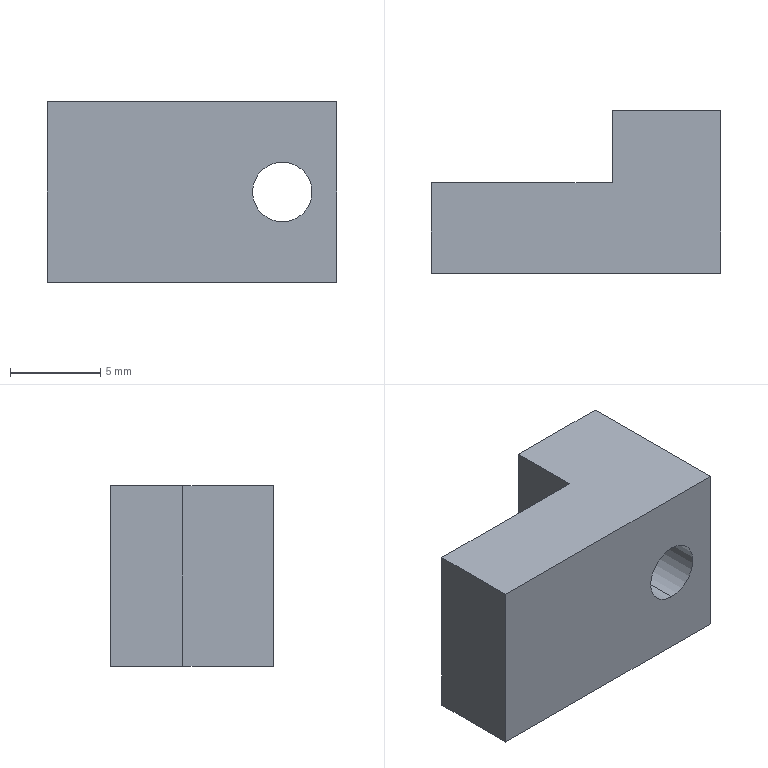Part | STEP file | limit block-1 | 1 solid | 13 faces | box 16 x 9 x 10 mm | volume 904.118 mm3 | plane 9 | cylinder 4 | commonest cylinder face diameters 3.3 x2 5 x2
STEP:
#1=CARTESIAN_POINT('',(0.,0.,0.));
#2=DIRECTION('',(0.,0.,1.));
#3=DIRECTION('',(1.,0.,0.));
#4=AXIS2_PLACEMENT_3D('',#1,#2,#3);
#5=CARTESIAN_POINT('',(5.5,-3.,7.5));
#6=VERTEX_POINT('',#5);
#7=CARTESIAN_POINT('',(5.5,0.,7.5));
#8=VERTEX_POINT('',#7);
#9=CARTESIAN_POINT('',(5.5,-3.,7.5));
#10=DIRECTION('',(0.,1.,0.));
#11=VECTOR('',#10,1.);
#12=LINE('',#9,#11);
#13=CARTESIAN_POINT('',(5.5,-3.,5.));
#14=DIRECTION('',(0.,1.,0.));
#15=DIRECTION('',(0.,0.,1.));
#16=AXIS2_PLACEMENT_3D('',#13,#14,#15);
#17=CYLINDRICAL_SURFACE('',#16,2.5);
#18=CARTESIAN_POINT('',(6.283,0.));
#19=DIRECTION('',(0.,1.));
#20=VECTOR('',#19,1.);
#21=LINE('',#18,#20);
#22=(GEOMETRIC_REPRESENTATION_CONTEXT(2)PARAMETRIC_REPRESENTATION_CONTEXT()REPRESENTATION_CONTEXT('',''));
#23=DEFINITIONAL_REPRESENTATION('',(#21),#22);
#24=PCURVE('',#17,#23);
#25=CARTESIAN_POINT('',(5.5,-3.,5.));
#26=DIRECTION('',(0.,1.,0.));
#27=DIRECTION('',(0.,0.,1.));
#28=AXIS2_PLACEMENT_3D('',#25,#26,#27);
#29=CYLINDRICAL_SURFACE('',#28,2.5);
#30=CARTESIAN_POINT('',(0.,0.));
#31=DIRECTION('',(0.,1.));
#32=VECTOR('',#31,1.);
#33=LINE('',#30,#32);
#34=(GEOMETRIC_REPRESENTATION_CONTEXT(2)PARAMETRIC_REPRESENTATION_CONTEXT()REPRESENTATION_CONTEXT('',''));
#35=DEFINITIONAL_REPRESENTATION('',(#33),#34);
#36=PCURVE('',#29,#35);
#37=SURFACE_CURVE('',#12,(#24,#36),.PCURVE_S1.);
#38=EDGE_CURVE('',#6,#8,#37,.T.);
#39=ORIENTED_EDGE('',*,*,#38,.T.);
#40=CARTESIAN_POINT('',(5.5,0.,2.5));
#41=VERTEX_POINT('',#40);
#42=CARTESIAN_POINT('',(5.5,0.,5.));
#43=DIRECTION('',(0.,1.,0.));
#44=DIRECTION('',(0.,0.,1.));
#45=AXIS2_PLACEMENT_3D('',#42,#43,#44);
#46=CIRCLE('',#45,2.5);
#47=CARTESIAN_POINT('',(0.,3.));
#48=DIRECTION('',(1.,0.));
#49=VECTOR('',#48,1.);
#50=LINE('',#47,#49);
#51=(GEOMETRIC_REPRESENTATION_CONTEXT(2)PARAMETRIC_REPRESENTATION_CONTEXT()REPRESENTATION_CONTEXT('',''));
#52=DEFINITIONAL_REPRESENTATION('',(#50),#51);
#53=PCURVE('',#17,#52);
#54=CARTESIAN_POINT('',(0.,0.,10.));
#55=DIRECTION('',(0.,-1.,0.));
#56=DIRECTION('',(0.,0.,-1.));
#57=AXIS2_PLACEMENT_3D('',#54,#55,#56);
#58=PLANE('',#57);
#59=CARTESIAN_POINT('',(2.5,5.5));
#60=CARTESIAN_POINT('',(2.5,9.83));
#61=CARTESIAN_POINT('',(6.25,7.665));
#62=CARTESIAN_POINT('',(10.,5.5));
#63=CARTESIAN_POINT('',(6.25,3.335));
#64=CARTESIAN_POINT('',(2.5,1.17));
#65=CARTESIAN_POINT('',(2.5,5.5));
#66=(BOUNDED_CURVE()B_SPLINE_CURVE(2,(#59,#60,#61,#62,#63,#64,#65),.UNSPECIFIED.,.T.,.F.)B_SPLINE_CURVE_WITH_KNOTS((1,2,2,2,2,1),(-2.094,0.,2.094,4.189,6.283,8.378),.UNSPECIFIED.)CURVE()GEOMETRIC_REPRESENTATION_ITEM()RATIONAL_B_SPLINE_CURVE((1.,0.5,1.,0.5,1.,0.5,1.))REPRESENTATION_ITEM(''));
#67=(GEOMETRIC_REPRESENTATION_CONTEXT(2)PARAMETRIC_REPRESENTATION_CONTEXT()REPRESENTATION_CONTEXT('',''));
#68=DEFINITIONAL_REPRESENTATION('',(#66),#67);
#69=PCURVE('',#58,#68);
#70=SURFACE_CURVE('',#46,(#53,#69),.PCURVE_S1.);
#71=EDGE_CURVE('',#41,#8,#70,.T.);
#72=ORIENTED_EDGE('',*,*,#71,.F.);
#73=CARTESIAN_POINT('',(5.5,-3.,2.5));
#74=VERTEX_POINT('',#73);
#75=CARTESIAN_POINT('',(5.5,-3.,2.5));
#76=DIRECTION('',(0.,1.,0.));
#77=VECTOR('',#76,1.);
#78=LINE('',#75,#77);
#79=CARTESIAN_POINT('',(3.142,0.));
#80=DIRECTION('',(0.,1.));
#81=VECTOR('',#80,1.);
#82=LINE('',#79,#81);
#83=(GEOMETRIC_REPRESENTATION_CONTEXT(2)PARAMETRIC_REPRESENTATION_CONTEXT()REPRESENTATION_CONTEXT('',''));
#84=DEFINITIONAL_REPRESENTATION('',(#82),#83);
#85=PCURVE('',#17,#84);
#86=CARTESIAN_POINT('',(3.142,0.));
#87=DIRECTION('',(0.,1.));
#88=VECTOR('',#87,1.);
#89=LINE('',#86,#88);
#90=(GEOMETRIC_REPRESENTATION_CONTEXT(2)PARAMETRIC_REPRESENTATION_CONTEXT()REPRESENTATION_CONTEXT('',''));
#91=DEFINITIONAL_REPRESENTATION('',(#89),#90);
#92=PCURVE('',#29,#91);
#93=SURFACE_CURVE('',#78,(#85,#92),.PCURVE_S1.);
#94=EDGE_CURVE('',#74,#41,#93,.T.);
#95=ORIENTED_EDGE('',*,*,#94,.F.);
#96=CARTESIAN_POINT('',(5.5,-3.,5.));
#97=DIRECTION('',(0.,1.,0.));
#98=DIRECTION('',(0.,0.,1.));
#99=AXIS2_PLACEMENT_3D('',#96,#97,#98);
#100=CIRCLE('',#99,2.5);
#101=CARTESIAN_POINT('',(0.,0.));
#102=DIRECTION('',(1.,0.));
#103=VECTOR('',#102,1.);
#104=LINE('',#101,#103);
#105=(GEOMETRIC_REPRESENTATION_CONTEXT(2)PARAMETRIC_REPRESENTATION_CONTEXT()REPRESENTATION_CONTEXT('',''));
#106=DEFINITIONAL_REPRESENTATION('',(#104),#105);
#107=PCURVE('',#17,#106);
#108=CARTESIAN_POINT('',(5.5,-3.,5.));
#109=DIRECTION('',(0.,1.,0.));
#110=DIRECTION('',(0.,0.,1.));
#111=AXIS2_PLACEMENT_3D('',#108,#109,#110);
#112=PLANE('',#111);
#113=CARTESIAN_POINT('',(0.,0.));
#114=DIRECTION('',(1.,0.));
#115=AXIS2_PLACEMENT_2D('',#113,#114);
#116=CIRCLE('',#115,2.5);
#117=(GEOMETRIC_REPRESENTATION_CONTEXT(2)PARAMETRIC_REPRESENTATION_CONTEXT()REPRESENTATION_CONTEXT('',''));
#118=DEFINITIONAL_REPRESENTATION('',(#116),#117);
#119=PCURVE('',#112,#118);
#120=SURFACE_CURVE('',#100,(#107,#119),.PCURVE_S1.);
#121=EDGE_CURVE('',#74,#6,#120,.T.);
#122=ORIENTED_EDGE('',*,*,#121,.T.);
#123=EDGE_LOOP('',(#39,#72,#95,#122));
#124=FACE_BOUND('',#123,.F.);
#125=ADVANCED_FACE('',(#124),#17,.F.);
#126=CARTESIAN_POINT('',(15.,-5.,6.65));
#127=VERTEX_POINT('',#126);
#128=CARTESIAN_POINT('',(15.,4.,6.65));
#129=VERTEX_POINT('',#128);
#130=CARTESIAN_POINT('',(15.,4.,6.65));
#131=DIRECTION('',(0.,1.,0.));
#132=VECTOR('',#131,1.);
#133=LINE('',#130,#132);
#134=CARTESIAN_POINT('',(15.,4.,5.));
#135=DIRECTION('',(0.,1.,0.));
#136=DIRECTION('',(0.,0.,1.));
#137=AXIS2_PLACEMENT_3D('',#134,#135,#136);
#138=CYLINDRICAL_SURFACE('',#137,1.65);
#139=CARTESIAN_POINT('',(6.283,0.));
#140=DIRECTION('',(0.,1.));
#141=VECTOR('',#140,1.);
#142=LINE('',#139,#141);
#143=(GEOMETRIC_REPRESENTATION_CONTEXT(2)PARAMETRIC_REPRESENTATION_CONTEXT()REPRESENTATION_CONTEXT('',''));
#144=DEFINITIONAL_REPRESENTATION('',(#142),#143);
#145=PCURVE('',#138,#144);
#146=CARTESIAN_POINT('',(15.,4.,5.));
#147=DIRECTION('',(0.,1.,0.));
#148=DIRECTION('',(0.,0.,1.));
#149=AXIS2_PLACEMENT_3D('',#146,#147,#148);
#150=CYLINDRICAL_SURFACE('',#149,1.65);
#151=CARTESIAN_POINT('',(0.,0.));
#152=DIRECTION('',(0.,1.));
#153=VECTOR('',#152,1.);
#154=LINE('',#151,#153);
#155=(GEOMETRIC_REPRESENTATION_CONTEXT(2)PARAMETRIC_REPRESENTATION_CONTEXT()REPRESENTATION_CONTEXT('',''));
#156=DEFINITIONAL_REPRESENTATION('',(#154),#155);
#157=PCURVE('',#150,#156);
#158=SURFACE_CURVE('',#133,(#145,#157),.PCURVE_S1.);
#159=EDGE_CURVE('',#127,#129,#158,.T.);
#160=ORIENTED_EDGE('',*,*,#159,.T.);
#161=CARTESIAN_POINT('',(15.,4.,3.35));
#162=VERTEX_POINT('',#161);
#163=CARTESIAN_POINT('',(15.,4.,5.));
#164=DIRECTION('',(0.,1.,0.));
#165=DIRECTION('',(0.,0.,1.));
#166=AXIS2_PLACEMENT_3D('',#163,#164,#165);
#167=CIRCLE('',#166,1.65);
#168=CARTESIAN_POINT('',(0.,0.));
#169=DIRECTION('',(1.,0.));
#170=VECTOR('',#169,1.);
#171=LINE('',#168,#170);
#172=(GEOMETRIC_REPRESENTATION_CONTEXT(2)PARAMETRIC_REPRESENTATION_CONTEXT()REPRESENTATION_CONTEXT('',''));
#173=DEFINITIONAL_REPRESENTATION('',(#171),#172);
#174=PCURVE('',#138,#173);
#175=CARTESIAN_POINT('',(12.,4.,10.));
#176=DIRECTION('',(0.,-1.,0.));
#177=DIRECTION('',(0.,0.,-1.));
#178=AXIS2_PLACEMENT_3D('',#175,#176,#177);
#179=PLANE('',#178);
#180=CARTESIAN_POINT('',(3.35,3.));
#181=CARTESIAN_POINT('',(3.35,5.858));
#182=CARTESIAN_POINT('',(5.825,4.429));
#183=CARTESIAN_POINT('',(8.3,3.));
#184=CARTESIAN_POINT('',(5.825,1.571));
#185=CARTESIAN_POINT('',(3.35,0.1421));
#186=CARTESIAN_POINT('',(3.35,3.));
#187=(BOUNDED_CURVE()B_SPLINE_CURVE(2,(#180,#181,#182,#183,#184,#185,#186),.UNSPECIFIED.,.T.,.F.)B_SPLINE_CURVE_WITH_KNOTS((1,2,2,2,2,1),(-2.094,0.,2.094,4.189,6.283,8.378),.UNSPECIFIED.)CURVE()GEOMETRIC_REPRESENTATION_ITEM()RATIONAL_B_SPLINE_CURVE((1.,0.5,1.,0.5,1.,0.5,1.))REPRESENTATION_ITEM(''));
#188=(GEOMETRIC_REPRESENTATION_CONTEXT(2)PARAMETRIC_REPRESENTATION_CONTEXT()REPRESENTATION_CONTEXT('',''));
#189=DEFINITIONAL_REPRESENTATION('',(#187),#188);
#190=PCURVE('',#179,#189);
#191=SURFACE_CURVE('',#167,(#174,#190),.PCURVE_S1.);
#192=EDGE_CURVE('',#162,#129,#191,.T.);
#193=ORIENTED_EDGE('',*,*,#192,.F.);
#194=CARTESIAN_POINT('',(15.,-5.,3.35));
#195=VERTEX_POINT('',#194);
#196=CARTESIAN_POINT('',(15.,4.,3.35));
#197=DIRECTION('',(0.,1.,0.));
#198=VECTOR('',#197,1.);
#199=LINE('',#196,#198);
#200=CARTESIAN_POINT('',(3.142,0.));
#201=DIRECTION('',(0.,1.));
#202=VECTOR('',#201,1.);
#203=LINE('',#200,#202);
#204=(GEOMETRIC_REPRESENTATION_CONTEXT(2)PARAMETRIC_REPRESENTATION_CONTEXT()REPRESENTATION_CONTEXT('',''));
#205=DEFINITIONAL_REPRESENTATION('',(#203),#204);
#206=PCURVE('',#138,#205);
#207=CARTESIAN_POINT('',(3.142,0.));
#208=DIRECTION('',(0.,1.));
#209=VECTOR('',#208,1.);
#210=LINE('',#207,#209);
#211=(GEOMETRIC_REPRESENTATION_CONTEXT(2)PARAMETRIC_REPRESENTATION_CONTEXT()REPRESENTATION_CONTEXT('',''));
#212=DEFINITIONAL_REPRESENTATION('',(#210),#211);
#213=PCURVE('',#150,#212);
#214=SURFACE_CURVE('',#199,(#206,#213),.PCURVE_S1.);
#215=EDGE_CURVE('',#195,#162,#214,.T.);
#216=ORIENTED_EDGE('',*,*,#215,.F.);
#217=CARTESIAN_POINT('',(15.,-5.,5.));
#218=DIRECTION('',(0.,1.,0.));
#219=DIRECTION('',(0.,0.,1.));
#220=AXIS2_PLACEMENT_3D('',#217,#218,#219);
#221=CIRCLE('',#220,1.65);
#222=CARTESIAN_POINT('',(0.,-9.));
#223=DIRECTION('',(1.,0.));
#224=VECTOR('',#223,1.);
#225=LINE('',#222,#224);
#226=(GEOMETRIC_REPRESENTATION_CONTEXT(2)PARAMETRIC_REPRESENTATION_CONTEXT()REPRESENTATION_CONTEXT('',''));
#227=DEFINITIONAL_REPRESENTATION('',(#225),#226);
#228=PCURVE('',#138,#227);
#229=CARTESIAN_POINT('',(18.,-5.,10.));
#230=DIRECTION('',(0.,1.,0.));
#231=DIRECTION('',(-1.,0.,0.));
#232=AXIS2_PLACEMENT_3D('',#229,#230,#231);
#233=PLANE('',#232);
#234=CARTESIAN_POINT('',(3.,-5.));
#235=DIRECTION('',(0.,1.));
#236=AXIS2_PLACEMENT_2D('',#234,#235);
#237=CIRCLE('',#236,1.65);
#238=(GEOMETRIC_REPRESENTATION_CONTEXT(2)PARAMETRIC_REPRESENTATION_CONTEXT()REPRESENTATION_CONTEXT('',''));
#239=DEFINITIONAL_REPRESENTATION('',(#237),#238);
#240=PCURVE('',#233,#239);
#241=SURFACE_CURVE('',#221,(#228,#240),.PCURVE_S1.);
#242=EDGE_CURVE('',#195,#127,#241,.T.);
#243=ORIENTED_EDGE('',*,*,#242,.T.);
#244=EDGE_LOOP('',(#160,#193,#216,#243));
#245=FACE_BOUND('',#244,.F.);
#246=ADVANCED_FACE('',(#245),#138,.F.);
#247=CARTESIAN_POINT('',(15.,-5.,5.));
#248=DIRECTION('',(0.,1.,0.));
#249=DIRECTION('',(0.,0.,1.));
#250=AXIS2_PLACEMENT_3D('',#247,#248,#249);
#251=CIRCLE('',#250,1.65);
#252=CARTESIAN_POINT('',(3.,-5.));
#253=DIRECTION('',(0.,1.));
#254=AXIS2_PLACEMENT_2D('',#252,#253);
#255=CIRCLE('',#254,1.65);
#256=(GEOMETRIC_REPRESENTATION_CONTEXT(2)PARAMETRIC_REPRESENTATION_CONTEXT()REPRESENTATION_CONTEXT('',''));
#257=DEFINITIONAL_REPRESENTATION('',(#255),#256);
#258=PCURVE('',#233,#257);
#259=CARTESIAN_POINT('',(0.,-9.));
#260=DIRECTION('',(1.,0.));
#261=VECTOR('',#260,1.);
#262=LINE('',#259,#261);
#263=(GEOMETRIC_REPRESENTATION_CONTEXT(2)PARAMETRIC_REPRESENTATION_CONTEXT()REPRESENTATION_CONTEXT('',''));
#264=DEFINITIONAL_REPRESENTATION('',(#262),#263);
#265=PCURVE('',#150,#264);
#266=SURFACE_CURVE('',#251,(#258,#265),.PCURVE_S1.);
#267=EDGE_CURVE('',#127,#195,#266,.T.);
#268=ORIENTED_EDGE('',*,*,#267,.T.);
#269=ORIENTED_EDGE('',*,*,#242,.T.);
#270=EDGE_LOOP('',(#268,#269));
#271=FACE_BOUND('',#270,.T.);
#272=CARTESIAN_POINT('',(2.,-5.,10.));
#273=VERTEX_POINT('',#272);
#274=CARTESIAN_POINT('',(18.,-5.,10.));
#275=VERTEX_POINT('',#274);
#276=CARTESIAN_POINT('',(18.,-5.,10.));
#277=DIRECTION('',(1.,0.,0.));
#278=VECTOR('',#277,1.);
#279=LINE('',#276,#278);
#280=CARTESIAN_POINT('',(0.,0.));
#281=DIRECTION('',(-1.,0.));
#282=VECTOR('',#281,1.);
#283=LINE('',#280,#282);
#284=(GEOMETRIC_REPRESENTATION_CONTEXT(2)PARAMETRIC_REPRESENTATION_CONTEXT()REPRESENTATION_CONTEXT('',''));
#285=DEFINITIONAL_REPRESENTATION('',(#283),#284);
#286=PCURVE('',#233,#285);
#287=CARTESIAN_POINT('',(0.,0.,10.));
#288=DIRECTION('',(0.,0.,-1.));
#289=DIRECTION('',(-1.,0.,0.));
#290=AXIS2_PLACEMENT_3D('',#287,#288,#289);
#291=PLANE('',#290);
#292=CARTESIAN_POINT('',(-18.,-5.));
#293=DIRECTION('',(-1.,0.));
#294=VECTOR('',#293,1.);
#295=LINE('',#292,#294);
#296=(GEOMETRIC_REPRESENTATION_CONTEXT(2)PARAMETRIC_REPRESENTATION_CONTEXT()REPRESENTATION_CONTEXT('',''));
#297=DEFINITIONAL_REPRESENTATION('',(#295),#296);
#298=PCURVE('',#291,#297);
#299=SURFACE_CURVE('',#279,(#286,#298),.PCURVE_S1.);
#300=EDGE_CURVE('',#273,#275,#299,.T.);
#301=ORIENTED_EDGE('',*,*,#300,.F.);
#302=CARTESIAN_POINT('',(2.,-5.,0.));
#303=VERTEX_POINT('',#302);
#304=CARTESIAN_POINT('',(2.,-5.,0.));
#305=DIRECTION('',(0.,0.,-1.));
#306=VECTOR('',#305,1.);
#307=LINE('',#304,#306);
#308=CARTESIAN_POINT('',(16.,-10.));
#309=DIRECTION('',(0.,-1.));
#310=VECTOR('',#309,1.);
#311=LINE('',#308,#310);
#312=(GEOMETRIC_REPRESENTATION_CONTEXT(2)PARAMETRIC_REPRESENTATION_CONTEXT()REPRESENTATION_CONTEXT('',''));
#313=DEFINITIONAL_REPRESENTATION('',(#311),#312);
#314=PCURVE('',#233,#313);
#315=CARTESIAN_POINT('',(2.,-5.,0.));
#316=DIRECTION('',(1.,0.,0.));
#317=DIRECTION('',(0.,0.,-1.));
#318=AXIS2_PLACEMENT_3D('',#315,#316,#317);
#319=PLANE('',#318);
#320=CARTESIAN_POINT('',(0.,0.));
#321=DIRECTION('',(1.,0.));
#322=VECTOR('',#321,1.);
#323=LINE('',#320,#322);
#324=(GEOMETRIC_REPRESENTATION_CONTEXT(2)PARAMETRIC_REPRESENTATION_CONTEXT()REPRESENTATION_CONTEXT('',''));
#325=DEFINITIONAL_REPRESENTATION('',(#323),#324);
#326=PCURVE('',#319,#325);
#327=SURFACE_CURVE('',#307,(#314,#326),.PCURVE_S1.);
#328=EDGE_CURVE('',#273,#303,#327,.T.);
#329=ORIENTED_EDGE('',*,*,#328,.T.);
#330=CARTESIAN_POINT('',(18.,-5.,0.));
#331=VERTEX_POINT('',#330);
#332=CARTESIAN_POINT('',(18.,-5.,0.));
#333=DIRECTION('',(1.,0.,0.));
#334=VECTOR('',#333,1.);
#335=LINE('',#332,#334);
#336=CARTESIAN_POINT('',(0.,-10.));
#337=DIRECTION('',(-1.,0.));
#338=VECTOR('',#337,1.);
#339=LINE('',#336,#338);
#340=(GEOMETRIC_REPRESENTATION_CONTEXT(2)PARAMETRIC_REPRESENTATION_CONTEXT()REPRESENTATION_CONTEXT('',''));
#341=DEFINITIONAL_REPRESENTATION('',(#339),#340);
#342=PCURVE('',#233,#341);
#343=CARTESIAN_POINT('',(0.,0.,0.));
#344=DIRECTION('',(0.,0.,-1.));
#345=DIRECTION('',(-1.,0.,0.));
#346=AXIS2_PLACEMENT_3D('',#343,#344,#345);
#347=PLANE('',#346);
#348=CARTESIAN_POINT('',(-18.,-5.));
#349=DIRECTION('',(-1.,0.));
#350=VECTOR('',#349,1.);
#351=LINE('',#348,#350);
#352=(GEOMETRIC_REPRESENTATION_CONTEXT(2)PARAMETRIC_REPRESENTATION_CONTEXT()REPRESENTATION_CONTEXT('',''));
#353=DEFINITIONAL_REPRESENTATION('',(#351),#352);
#354=PCURVE('',#347,#353);
#355=SURFACE_CURVE('',#335,(#342,#354),.PCURVE_S1.);
#356=EDGE_CURVE('',#303,#331,#355,.T.);
#357=ORIENTED_EDGE('',*,*,#356,.T.);
#358=CARTESIAN_POINT('',(18.,-5.,10.));
#359=DIRECTION('',(0.,0.,-1.));
#360=VECTOR('',#359,1.);
#361=LINE('',#358,#360);
#362=CARTESIAN_POINT('',(0.,0.));
#363=DIRECTION('',(0.,-1.));
#364=VECTOR('',#363,1.);
#365=LINE('',#362,#364);
#366=(GEOMETRIC_REPRESENTATION_CONTEXT(2)PARAMETRIC_REPRESENTATION_CONTEXT()REPRESENTATION_CONTEXT('',''));
#367=DEFINITIONAL_REPRESENTATION('',(#365),#366);
#368=PCURVE('',#233,#367);
#369=CARTESIAN_POINT('',(18.,4.,10.));
#370=DIRECTION('',(-1.,0.,0.));
#371=DIRECTION('',(0.,0.,1.));
#372=AXIS2_PLACEMENT_3D('',#369,#370,#371);
#373=PLANE('',#372);
#374=CARTESIAN_POINT('',(0.,-9.));
#375=DIRECTION('',(-1.,0.));
#376=VECTOR('',#375,1.);
#377=LINE('',#374,#376);
#378=(GEOMETRIC_REPRESENTATION_CONTEXT(2)PARAMETRIC_REPRESENTATION_CONTEXT()REPRESENTATION_CONTEXT('',''));
#379=DEFINITIONAL_REPRESENTATION('',(#377),#378);
#380=PCURVE('',#373,#379);
#381=SURFACE_CURVE('',#361,(#368,#380),.PCURVE_S1.);
#382=EDGE_CURVE('',#275,#331,#381,.T.);
#383=ORIENTED_EDGE('',*,*,#382,.F.);
#384=EDGE_LOOP('',(#301,#329,#357,#383));
#385=FACE_BOUND('',#384,.T.);
#386=ADVANCED_FACE('',(#271,#385),#233,.F.);
#387=CARTESIAN_POINT('',(18.,4.,0.));
#388=VERTEX_POINT('',#387);
#389=CARTESIAN_POINT('',(18.,4.,0.));
#390=DIRECTION('',(0.,1.,0.));
#391=VECTOR('',#390,1.);
#392=LINE('',#389,#391);
#393=CARTESIAN_POINT('',(-10.,0.));
#394=DIRECTION('',(0.,1.));
#395=VECTOR('',#394,1.);
#396=LINE('',#393,#395);
#397=(GEOMETRIC_REPRESENTATION_CONTEXT(2)PARAMETRIC_REPRESENTATION_CONTEXT()REPRESENTATION_CONTEXT('',''));
#398=DEFINITIONAL_REPRESENTATION('',(#396),#397);
#399=PCURVE('',#373,#398);
#400=CARTESIAN_POINT('',(-18.,4.));
#401=DIRECTION('',(0.,1.));
#402=VECTOR('',#401,1.);
#403=LINE('',#400,#402);
#404=(GEOMETRIC_REPRESENTATION_CONTEXT(2)PARAMETRIC_REPRESENTATION_CONTEXT()REPRESENTATION_CONTEXT('',''));
#405=DEFINITIONAL_REPRESENTATION('',(#403),#404);
#406=PCURVE('',#347,#405);
#407=SURFACE_CURVE('',#392,(#399,#406),.PCURVE_S1.);
#408=EDGE_CURVE('',#331,#388,#407,.T.);
#409=ORIENTED_EDGE('',*,*,#408,.T.);
#410=CARTESIAN_POINT('',(18.,4.,10.));
#411=VERTEX_POINT('',#410);
#412=CARTESIAN_POINT('',(18.,4.,10.));
#413=DIRECTION('',(0.,0.,-1.));
#414=VECTOR('',#413,1.);
#415=LINE('',#412,#414);
#416=CARTESIAN_POINT('',(0.,0.));
#417=DIRECTION('',(-1.,0.));
#418=VECTOR('',#417,1.);
#419=LINE('',#416,#418);
#420=(GEOMETRIC_REPRESENTATION_CONTEXT(2)PARAMETRIC_REPRESENTATION_CONTEXT()REPRESENTATION_CONTEXT('',''));
#421=DEFINITIONAL_REPRESENTATION('',(#419),#420);
#422=PCURVE('',#373,#421);
#423=CARTESIAN_POINT('',(0.,6.));
#424=DIRECTION('',(1.,0.));
#425=VECTOR('',#424,1.);
#426=LINE('',#423,#425);
#427=(GEOMETRIC_REPRESENTATION_CONTEXT(2)PARAMETRIC_REPRESENTATION_CONTEXT()REPRESENTATION_CONTEXT('',''));
#428=DEFINITIONAL_REPRESENTATION('',(#426),#427);
#429=PCURVE('',#179,#428);
#430=SURFACE_CURVE('',#415,(#422,#429),.PCURVE_S1.);
#431=EDGE_CURVE('',#411,#388,#430,.T.);
#432=ORIENTED_EDGE('',*,*,#431,.F.);
#433=CARTESIAN_POINT('',(18.,4.,10.));
#434=DIRECTION('',(0.,1.,0.));
#435=VECTOR('',#434,1.);
#436=LINE('',#433,#435);
#437=CARTESIAN_POINT('',(0.,0.));
#438=DIRECTION('',(0.,1.));
#439=VECTOR('',#438,1.);
#440=LINE('',#437,#439);
#441=(GEOMETRIC_REPRESENTATION_CONTEXT(2)PARAMETRIC_REPRESENTATION_CONTEXT()REPRESENTATION_CONTEXT('',''));
#442=DEFINITIONAL_REPRESENTATION('',(#440),#441);
#443=PCURVE('',#373,#442);
#444=CARTESIAN_POINT('',(-18.,4.));
#445=DIRECTION('',(0.,1.));
#446=VECTOR('',#445,1.);
#447=LINE('',#444,#446);
#448=(GEOMETRIC_REPRESENTATION_CONTEXT(2)PARAMETRIC_REPRESENTATION_CONTEXT()REPRESENTATION_CONTEXT('',''));
#449=DEFINITIONAL_REPRESENTATION('',(#447),#448);
#450=PCURVE('',#291,#449);
#451=SURFACE_CURVE('',#436,(#443,#450),.PCURVE_S1.);
#452=EDGE_CURVE('',#275,#411,#451,.T.);
#453=ORIENTED_EDGE('',*,*,#452,.F.);
#454=ORIENTED_EDGE('',*,*,#382,.T.);
#455=EDGE_LOOP('',(#409,#432,#453,#454));
#456=FACE_BOUND('',#455,.T.);
#457=ADVANCED_FACE('',(#456),#373,.F.);
#458=CARTESIAN_POINT('',(15.,4.,5.));
#459=DIRECTION('',(0.,1.,0.));
#460=DIRECTION('',(0.,0.,1.));
#461=AXIS2_PLACEMENT_3D('',#458,#459,#460);
#462=CIRCLE('',#461,1.65);
#463=CARTESIAN_POINT('',(3.35,3.));
#464=CARTESIAN_POINT('',(3.35,5.858));
#465=CARTESIAN_POINT('',(5.825,4.429));
#466=CARTESIAN_POINT('',(8.3,3.));
#467=CARTESIAN_POINT('',(5.825,1.571));
#468=CARTESIAN_POINT('',(3.35,0.1421));
#469=CARTESIAN_POINT('',(3.35,3.));
#470=(BOUNDED_CURVE()B_SPLINE_CURVE(2,(#463,#464,#465,#466,#467,#468,#469),.UNSPECIFIED.,.T.,.F.)B_SPLINE_CURVE_WITH_KNOTS((1,2,2,2,2,1),(-2.094,0.,2.094,4.189,6.283,8.378),.UNSPECIFIED.)CURVE()GEOMETRIC_REPRESENTATION_ITEM()RATIONAL_B_SPLINE_CURVE((1.,0.5,1.,0.5,1.,0.5,1.))REPRESENTATION_ITEM(''));
#471=(GEOMETRIC_REPRESENTATION_CONTEXT(2)PARAMETRIC_REPRESENTATION_CONTEXT()REPRESENTATION_CONTEXT('',''));
#472=DEFINITIONAL_REPRESENTATION('',(#470),#471);
#473=PCURVE('',#179,#472);
#474=CARTESIAN_POINT('',(0.,0.));
#475=DIRECTION('',(1.,0.));
#476=VECTOR('',#475,1.);
#477=LINE('',#474,#476);
#478=(GEOMETRIC_REPRESENTATION_CONTEXT(2)PARAMETRIC_REPRESENTATION_CONTEXT()REPRESENTATION_CONTEXT('',''));
#479=DEFINITIONAL_REPRESENTATION('',(#477),#478);
#480=PCURVE('',#150,#479);
#481=SURFACE_CURVE('',#462,(#473,#480),.PCURVE_S1.);
#482=EDGE_CURVE('',#129,#162,#481,.T.);
#483=ORIENTED_EDGE('',*,*,#482,.F.);
#484=ORIENTED_EDGE('',*,*,#192,.F.);
#485=EDGE_LOOP('',(#483,#484));
#486=FACE_BOUND('',#485,.T.);
#487=CARTESIAN_POINT('',(12.,4.,0.));
#488=VERTEX_POINT('',#487);
#489=CARTESIAN_POINT('',(12.,4.,0.));
#490=DIRECTION('',(-1.,0.,0.));
#491=VECTOR('',#490,1.);
#492=LINE('',#489,#491);
#493=CARTESIAN_POINT('',(10.,0.));
#494=DIRECTION('',(0.,-1.));
#495=VECTOR('',#494,1.);
#496=LINE('',#493,#495);
#497=(GEOMETRIC_REPRESENTATION_CONTEXT(2)PARAMETRIC_REPRESENTATION_CONTEXT()REPRESENTATION_CONTEXT('',''));
#498=DEFINITIONAL_REPRESENTATION('',(#496),#497);
#499=PCURVE('',#179,#498);
#500=CARTESIAN_POINT('',(-12.,4.));
#501=DIRECTION('',(1.,0.));
#502=VECTOR('',#501,1.);
#503=LINE('',#500,#502);
#504=(GEOMETRIC_REPRESENTATION_CONTEXT(2)PARAMETRIC_REPRESENTATION_CONTEXT()REPRESENTATION_CONTEXT('',''));
#505=DEFINITIONAL_REPRESENTATION('',(#503),#504);
#506=PCURVE('',#347,#505);
#507=SURFACE_CURVE('',#492,(#499,#506),.PCURVE_S1.);
#508=EDGE_CURVE('',#388,#488,#507,.T.);
#509=ORIENTED_EDGE('',*,*,#508,.T.);
#510=CARTESIAN_POINT('',(12.,4.,10.));
#511=VERTEX_POINT('',#510);
#512=CARTESIAN_POINT('',(12.,4.,10.));
#513=DIRECTION('',(0.,0.,-1.));
#514=VECTOR('',#513,1.);
#515=LINE('',#512,#514);
#516=CARTESIAN_POINT('',(0.,0.));
#517=DIRECTION('',(1.,0.));
#518=VECTOR('',#517,1.);
#519=LINE('',#516,#518);
#520=(GEOMETRIC_REPRESENTATION_CONTEXT(2)PARAMETRIC_REPRESENTATION_CONTEXT()REPRESENTATION_CONTEXT('',''));
#521=DEFINITIONAL_REPRESENTATION('',(#519),#520);
#522=PCURVE('',#179,#521);
#523=CARTESIAN_POINT('',(12.,0.,10.));
#524=DIRECTION('',(1.,0.,0.));
#525=DIRECTION('',(0.,0.,-1.));
#526=AXIS2_PLACEMENT_3D('',#523,#524,#525);
#527=PLANE('',#526);
#528=CARTESIAN_POINT('',(0.,4.));
#529=DIRECTION('',(1.,0.));
#530=VECTOR('',#529,1.);
#531=LINE('',#528,#530);
#532=(GEOMETRIC_REPRESENTATION_CONTEXT(2)PARAMETRIC_REPRESENTATION_CONTEXT()REPRESENTATION_CONTEXT('',''));
#533=DEFINITIONAL_REPRESENTATION('',(#531),#532);
#534=PCURVE('',#527,#533);
#535=SURFACE_CURVE('',#515,(#522,#534),.PCURVE_S1.);
#536=EDGE_CURVE('',#511,#488,#535,.T.);
#537=ORIENTED_EDGE('',*,*,#536,.F.);
#538=CARTESIAN_POINT('',(12.,4.,10.));
#539=DIRECTION('',(-1.,0.,0.));
#540=VECTOR('',#539,1.);
#541=LINE('',#538,#540);
#542=CARTESIAN_POINT('',(0.,0.));
#543=DIRECTION('',(0.,-1.));
#544=VECTOR('',#543,1.);
#545=LINE('',#542,#544);
#546=(GEOMETRIC_REPRESENTATION_CONTEXT(2)PARAMETRIC_REPRESENTATION_CONTEXT()REPRESENTATION_CONTEXT('',''));
#547=DEFINITIONAL_REPRESENTATION('',(#545),#546);
#548=PCURVE('',#179,#547);
#549=CARTESIAN_POINT('',(-12.,4.));
#550=DIRECTION('',(1.,0.));
#551=VECTOR('',#550,1.);
#552=LINE('',#549,#551);
#553=(GEOMETRIC_REPRESENTATION_CONTEXT(2)PARAMETRIC_REPRESENTATION_CONTEXT()REPRESENTATION_CONTEXT('',''));
#554=DEFINITIONAL_REPRESENTATION('',(#552),#553);
#555=PCURVE('',#291,#554);
#556=SURFACE_CURVE('',#541,(#548,#555),.PCURVE_S1.);
#557=EDGE_CURVE('',#411,#511,#556,.T.);
#558=ORIENTED_EDGE('',*,*,#557,.F.);
#559=ORIENTED_EDGE('',*,*,#431,.T.);
#560=EDGE_LOOP('',(#509,#537,#558,#559));
#561=FACE_BOUND('',#560,.T.);
#562=ADVANCED_FACE('',(#486,#561),#179,.F.);
#563=CARTESIAN_POINT('',(12.,0.,0.));
#564=VERTEX_POINT('',#563);
#565=CARTESIAN_POINT('',(12.,0.,0.));
#566=DIRECTION('',(0.,-1.,0.));
#567=VECTOR('',#566,1.);
#568=LINE('',#565,#567);
#569=CARTESIAN_POINT('',(10.,0.));
#570=DIRECTION('',(0.,-1.));
#571=VECTOR('',#570,1.);
#572=LINE('',#569,#571);
#573=(GEOMETRIC_REPRESENTATION_CONTEXT(2)PARAMETRIC_REPRESENTATION_CONTEXT()REPRESENTATION_CONTEXT('',''));
#574=DEFINITIONAL_REPRESENTATION('',(#572),#573);
#575=PCURVE('',#527,#574);
#576=CARTESIAN_POINT('',(-12.,0.));
#577=DIRECTION('',(0.,-1.));
#578=VECTOR('',#577,1.);
#579=LINE('',#576,#578);
#580=(GEOMETRIC_REPRESENTATION_CONTEXT(2)PARAMETRIC_REPRESENTATION_CONTEXT()REPRESENTATION_CONTEXT('',''));
#581=DEFINITIONAL_REPRESENTATION('',(#579),#580);
#582=PCURVE('',#347,#581);
#583=SURFACE_CURVE('',#568,(#575,#582),.PCURVE_S1.);
#584=EDGE_CURVE('',#488,#564,#583,.T.);
#585=ORIENTED_EDGE('',*,*,#584,.T.);
#586=CARTESIAN_POINT('',(12.,0.,10.));
#587=VERTEX_POINT('',#586);
#588=CARTESIAN_POINT('',(12.,0.,10.));
#589=DIRECTION('',(0.,0.,-1.));
#590=VECTOR('',#589,1.);
#591=LINE('',#588,#590);
#592=CARTESIAN_POINT('',(0.,0.));
#593=DIRECTION('',(1.,0.));
#594=VECTOR('',#593,1.);
#595=LINE('',#592,#594);
#596=(GEOMETRIC_REPRESENTATION_CONTEXT(2)PARAMETRIC_REPRESENTATION_CONTEXT()REPRESENTATION_CONTEXT('',''));
#597=DEFINITIONAL_REPRESENTATION('',(#595),#596);
#598=PCURVE('',#527,#597);
#599=CARTESIAN_POINT('',(0.,12.));
#600=DIRECTION('',(1.,0.));
#601=VECTOR('',#600,1.);
#602=LINE('',#599,#601);
#603=(GEOMETRIC_REPRESENTATION_CONTEXT(2)PARAMETRIC_REPRESENTATION_CONTEXT()REPRESENTATION_CONTEXT('',''));
#604=DEFINITIONAL_REPRESENTATION('',(#602),#603);
#605=PCURVE('',#58,#604);
#606=SURFACE_CURVE('',#591,(#598,#605),.PCURVE_S1.);
#607=EDGE_CURVE('',#587,#564,#606,.T.);
#608=ORIENTED_EDGE('',*,*,#607,.F.);
#609=CARTESIAN_POINT('',(12.,0.,10.));
#610=DIRECTION('',(0.,-1.,0.));
#611=VECTOR('',#610,1.);
#612=LINE('',#609,#611);
#613=CARTESIAN_POINT('',(0.,0.));
#614=DIRECTION('',(0.,-1.));
#615=VECTOR('',#614,1.);
#616=LINE('',#613,#615);
#617=(GEOMETRIC_REPRESENTATION_CONTEXT(2)PARAMETRIC_REPRESENTATION_CONTEXT()REPRESENTATION_CONTEXT('',''));
#618=DEFINITIONAL_REPRESENTATION('',(#616),#617);
#619=PCURVE('',#527,#618);
#620=CARTESIAN_POINT('',(-12.,0.));
#621=DIRECTION('',(0.,-1.));
#622=VECTOR('',#621,1.);
#623=LINE('',#620,#622);
#624=(GEOMETRIC_REPRESENTATION_CONTEXT(2)PARAMETRIC_REPRESENTATION_CONTEXT()REPRESENTATION_CONTEXT('',''));
#625=DEFINITIONAL_REPRESENTATION('',(#623),#624);
#626=PCURVE('',#291,#625);
#627=SURFACE_CURVE('',#612,(#619,#626),.PCURVE_S1.);
#628=EDGE_CURVE('',#511,#587,#627,.T.);
#629=ORIENTED_EDGE('',*,*,#628,.F.);
#630=ORIENTED_EDGE('',*,*,#536,.T.);
#631=EDGE_LOOP('',(#585,#608,#629,#630));
#632=FACE_BOUND('',#631,.T.);
#633=ADVANCED_FACE('',(#632),#527,.F.);
#634=CARTESIAN_POINT('',(5.5,0.,5.));
#635=DIRECTION('',(0.,1.,0.));
#636=DIRECTION('',(0.,0.,1.));
#637=AXIS2_PLACEMENT_3D('',#634,#635,#636);
#638=CIRCLE('',#637,2.5);
#639=CARTESIAN_POINT('',(2.5,5.5));
#640=CARTESIAN_POINT('',(2.5,9.83));
#641=CARTESIAN_POINT('',(6.25,7.665));
#642=CARTESIAN_POINT('',(10.,5.5));
#643=CARTESIAN_POINT('',(6.25,3.335));
#644=CARTESIAN_POINT('',(2.5,1.17));
#645=CARTESIAN_POINT('',(2.5,5.5));
#646=(BOUNDED_CURVE()B_SPLINE_CURVE(2,(#639,#640,#641,#642,#643,#644,#645),.UNSPECIFIED.,.T.,.F.)B_SPLINE_CURVE_WITH_KNOTS((1,2,2,2,2,1),(-2.094,0.,2.094,4.189,6.283,8.378),.UNSPECIFIED.)CURVE()GEOMETRIC_REPRESENTATION_ITEM()RATIONAL_B_SPLINE_CURVE((1.,0.5,1.,0.5,1.,0.5,1.))REPRESENTATION_ITEM(''));
#647=(GEOMETRIC_REPRESENTATION_CONTEXT(2)PARAMETRIC_REPRESENTATION_CONTEXT()REPRESENTATION_CONTEXT('',''));
#648=DEFINITIONAL_REPRESENTATION('',(#646),#647);
#649=PCURVE('',#58,#648);
#650=CARTESIAN_POINT('',(0.,3.));
#651=DIRECTION('',(1.,0.));
#652=VECTOR('',#651,1.);
#653=LINE('',#650,#652);
#654=(GEOMETRIC_REPRESENTATION_CONTEXT(2)PARAMETRIC_REPRESENTATION_CONTEXT()REPRESENTATION_CONTEXT('',''));
#655=DEFINITIONAL_REPRESENTATION('',(#653),#654);
#656=PCURVE('',#29,#655);
#657=SURFACE_CURVE('',#638,(#649,#656),.PCURVE_S1.);
#658=EDGE_CURVE('',#8,#41,#657,.T.);
#659=ORIENTED_EDGE('',*,*,#658,.F.);
#660=ORIENTED_EDGE('',*,*,#71,.F.);
#661=EDGE_LOOP('',(#659,#660));
#662=FACE_BOUND('',#661,.T.);
#663=CARTESIAN_POINT('',(2.,0.,0.));
#664=VERTEX_POINT('',#663);
#665=CARTESIAN_POINT('',(0.,0.,0.));
#666=DIRECTION('',(-1.,0.,0.));
#667=VECTOR('',#666,1.);
#668=LINE('',#665,#667);
#669=CARTESIAN_POINT('',(10.,0.));
#670=DIRECTION('',(0.,-1.));
#671=VECTOR('',#670,1.);
#672=LINE('',#669,#671);
#673=(GEOMETRIC_REPRESENTATION_CONTEXT(2)PARAMETRIC_REPRESENTATION_CONTEXT()REPRESENTATION_CONTEXT('',''));
#674=DEFINITIONAL_REPRESENTATION('',(#672),#673);
#675=PCURVE('',#58,#674);
#676=CARTESIAN_POINT('',(0.,0.));
#677=DIRECTION('',(1.,0.));
#678=VECTOR('',#677,1.);
#679=LINE('',#676,#678);
#680=(GEOMETRIC_REPRESENTATION_CONTEXT(2)PARAMETRIC_REPRESENTATION_CONTEXT()REPRESENTATION_CONTEXT('',''));
#681=DEFINITIONAL_REPRESENTATION('',(#679),#680);
#682=PCURVE('',#347,#681);
#683=SURFACE_CURVE('',#668,(#675,#682),.PCURVE_S1.);
#684=EDGE_CURVE('',#564,#664,#683,.T.);
#685=ORIENTED_EDGE('',*,*,#684,.T.);
#686=CARTESIAN_POINT('',(2.,0.,10.));
#687=VERTEX_POINT('',#686);
#688=CARTESIAN_POINT('',(2.,0.,0.));
#689=DIRECTION('',(0.,0.,-1.));
#690=VECTOR('',#689,1.);
#691=LINE('',#688,#690);
#692=CARTESIAN_POINT('',(10.,2.));
#693=DIRECTION('',(1.,0.));
#694=VECTOR('',#693,1.);
#695=LINE('',#692,#694);
#696=(GEOMETRIC_REPRESENTATION_CONTEXT(2)PARAMETRIC_REPRESENTATION_CONTEXT()REPRESENTATION_CONTEXT('',''));
#697=DEFINITIONAL_REPRESENTATION('',(#695),#696);
#698=PCURVE('',#58,#697);
#699=CARTESIAN_POINT('',(0.,5.));
#700=DIRECTION('',(1.,0.));
#701=VECTOR('',#700,1.);
#702=LINE('',#699,#701);
#703=(GEOMETRIC_REPRESENTATION_CONTEXT(2)PARAMETRIC_REPRESENTATION_CONTEXT()REPRESENTATION_CONTEXT('',''));
#704=DEFINITIONAL_REPRESENTATION('',(#702),#703);
#705=PCURVE('',#319,#704);
#706=SURFACE_CURVE('',#691,(#698,#705),.PCURVE_S1.);
#707=EDGE_CURVE('',#687,#664,#706,.T.);
#708=ORIENTED_EDGE('',*,*,#707,.F.);
#709=CARTESIAN_POINT('',(0.,0.,10.));
#710=DIRECTION('',(-1.,0.,0.));
#711=VECTOR('',#710,1.);
#712=LINE('',#709,#711);
#713=CARTESIAN_POINT('',(0.,0.));
#714=DIRECTION('',(0.,-1.));
#715=VECTOR('',#714,1.);
#716=LINE('',#713,#715);
#717=(GEOMETRIC_REPRESENTATION_CONTEXT(2)PARAMETRIC_REPRESENTATION_CONTEXT()REPRESENTATION_CONTEXT('',''));
#718=DEFINITIONAL_REPRESENTATION('',(#716),#717);
#719=PCURVE('',#58,#718);
#720=CARTESIAN_POINT('',(0.,0.));
#721=DIRECTION('',(1.,0.));
#722=VECTOR('',#721,1.);
#723=LINE('',#720,#722);
#724=(GEOMETRIC_REPRESENTATION_CONTEXT(2)PARAMETRIC_REPRESENTATION_CONTEXT()REPRESENTATION_CONTEXT('',''));
#725=DEFINITIONAL_REPRESENTATION('',(#723),#724);
#726=PCURVE('',#291,#725);
#727=SURFACE_CURVE('',#712,(#719,#726),.PCURVE_S1.);
#728=EDGE_CURVE('',#587,#687,#727,.T.);
#729=ORIENTED_EDGE('',*,*,#728,.F.);
#730=ORIENTED_EDGE('',*,*,#607,.T.);
#731=EDGE_LOOP('',(#685,#708,#729,#730));
#732=FACE_BOUND('',#731,.T.);
#733=ADVANCED_FACE('',(#662,#732),#58,.F.);
#734=ORIENTED_EDGE('',*,*,#728,.T.);
#735=CARTESIAN_POINT('',(2.,-5.,10.));
#736=DIRECTION('',(0.,1.,0.));
#737=VECTOR('',#736,1.);
#738=LINE('',#735,#737);
#739=CARTESIAN_POINT('',(-2.,-5.));
#740=DIRECTION('',(0.,1.));
#741=VECTOR('',#740,1.);
#742=LINE('',#739,#741);
#743=(GEOMETRIC_REPRESENTATION_CONTEXT(2)PARAMETRIC_REPRESENTATION_CONTEXT()REPRESENTATION_CONTEXT('',''));
#744=DEFINITIONAL_REPRESENTATION('',(#742),#743);
#745=PCURVE('',#291,#744);
#746=CARTESIAN_POINT('',(-10.,0.));
#747=DIRECTION('',(0.,1.));
#748=VECTOR('',#747,1.);
#749=LINE('',#746,#748);
#750=(GEOMETRIC_REPRESENTATION_CONTEXT(2)PARAMETRIC_REPRESENTATION_CONTEXT()REPRESENTATION_CONTEXT('',''));
#751=DEFINITIONAL_REPRESENTATION('',(#749),#750);
#752=PCURVE('',#319,#751);
#753=SURFACE_CURVE('',#738,(#745,#752),.PCURVE_S1.);
#754=EDGE_CURVE('',#273,#687,#753,.T.);
#755=ORIENTED_EDGE('',*,*,#754,.F.);
#756=ORIENTED_EDGE('',*,*,#300,.T.);
#757=ORIENTED_EDGE('',*,*,#452,.T.);
#758=ORIENTED_EDGE('',*,*,#557,.T.);
#759=ORIENTED_EDGE('',*,*,#628,.T.);
#760=EDGE_LOOP('',(#734,#755,#756,#757,#758,#759));
#761=FACE_BOUND('',#760,.T.);
#762=ADVANCED_FACE('',(#761),#291,.F.);
#763=CARTESIAN_POINT('',(2.,-5.,0.));
#764=DIRECTION('',(0.,1.,0.));
#765=VECTOR('',#764,1.);
#766=LINE('',#763,#765);
#767=CARTESIAN_POINT('',(-2.,-5.));
#768=DIRECTION('',(0.,1.));
#769=VECTOR('',#768,1.);
#770=LINE('',#767,#769);
#771=(GEOMETRIC_REPRESENTATION_CONTEXT(2)PARAMETRIC_REPRESENTATION_CONTEXT()REPRESENTATION_CONTEXT('',''));
#772=DEFINITIONAL_REPRESENTATION('',(#770),#771);
#773=PCURVE('',#347,#772);
#774=CARTESIAN_POINT('',(0.,0.));
#775=DIRECTION('',(0.,1.));
#776=VECTOR('',#775,1.);
#777=LINE('',#774,#776);
#778=(GEOMETRIC_REPRESENTATION_CONTEXT(2)PARAMETRIC_REPRESENTATION_CONTEXT()REPRESENTATION_CONTEXT('',''));
#779=DEFINITIONAL_REPRESENTATION('',(#777),#778);
#780=PCURVE('',#319,#779);
#781=SURFACE_CURVE('',#766,(#773,#780),.PCURVE_S1.);
#782=EDGE_CURVE('',#303,#664,#781,.T.);
#783=ORIENTED_EDGE('',*,*,#782,.T.);
#784=ORIENTED_EDGE('',*,*,#684,.F.);
#785=ORIENTED_EDGE('',*,*,#584,.F.);
#786=ORIENTED_EDGE('',*,*,#508,.F.);
#787=ORIENTED_EDGE('',*,*,#408,.F.);
#788=ORIENTED_EDGE('',*,*,#356,.F.);
#789=EDGE_LOOP('',(#783,#784,#785,#786,#787,#788));
#790=FACE_BOUND('',#789,.T.);
#791=ADVANCED_FACE('',(#790),#347,.T.);
#792=ORIENTED_EDGE('',*,*,#707,.T.);
#793=ORIENTED_EDGE('',*,*,#782,.F.);
#794=ORIENTED_EDGE('',*,*,#328,.F.);
#795=ORIENTED_EDGE('',*,*,#754,.T.);
#796=EDGE_LOOP('',(#792,#793,#794,#795));
#797=FACE_BOUND('',#796,.T.);
#798=ADVANCED_FACE('',(#797),#319,.F.);
#799=ORIENTED_EDGE('',*,*,#482,.F.);
#800=ORIENTED_EDGE('',*,*,#159,.F.);
#801=ORIENTED_EDGE('',*,*,#267,.T.);
#802=ORIENTED_EDGE('',*,*,#215,.T.);
#803=EDGE_LOOP('',(#799,#800,#801,#802));
#804=FACE_BOUND('',#803,.F.);
#805=ADVANCED_FACE('',(#804),#150,.F.);
#806=ORIENTED_EDGE('',*,*,#658,.F.);
#807=ORIENTED_EDGE('',*,*,#38,.F.);
#808=CARTESIAN_POINT('',(5.5,-3.,5.));
#809=DIRECTION('',(0.,1.,0.));
#810=DIRECTION('',(0.,0.,1.));
#811=AXIS2_PLACEMENT_3D('',#808,#809,#810);
#812=CIRCLE('',#811,2.5);
#813=CARTESIAN_POINT('',(0.,0.));
#814=DIRECTION('',(1.,0.));
#815=VECTOR('',#814,1.);
#816=LINE('',#813,#815);
#817=(GEOMETRIC_REPRESENTATION_CONTEXT(2)PARAMETRIC_REPRESENTATION_CONTEXT()REPRESENTATION_CONTEXT('',''));
#818=DEFINITIONAL_REPRESENTATION('',(#816),#817);
#819=PCURVE('',#29,#818);
#820=CARTESIAN_POINT('',(0.,0.));
#821=DIRECTION('',(1.,0.));
#822=AXIS2_PLACEMENT_2D('',#820,#821);
#823=CIRCLE('',#822,2.5);
#824=(GEOMETRIC_REPRESENTATION_CONTEXT(2)PARAMETRIC_REPRESENTATION_CONTEXT()REPRESENTATION_CONTEXT('',''));
#825=DEFINITIONAL_REPRESENTATION('',(#823),#824);
#826=PCURVE('',#112,#825);
#827=SURFACE_CURVE('',#812,(#819,#826),.PCURVE_S1.);
#828=EDGE_CURVE('',#6,#74,#827,.T.);
#829=ORIENTED_EDGE('',*,*,#828,.T.);
#830=ORIENTED_EDGE('',*,*,#94,.T.);
#831=EDGE_LOOP('',(#806,#807,#829,#830));
#832=FACE_BOUND('',#831,.F.);
#833=ADVANCED_FACE('',(#832),#29,.F.);
#834=ORIENTED_EDGE('',*,*,#828,.T.);
#835=ORIENTED_EDGE('',*,*,#121,.T.);
#836=EDGE_LOOP('',(#834,#835));
#837=FACE_BOUND('',#836,.T.);
#838=ADVANCED_FACE('',(#837),#112,.T.);
#839=CLOSED_SHELL('',(#125,#246,#386,#457,#562,#633,#733,#762,#791,#798,#805,#833,#838));
#840=MANIFOLD_SOLID_BREP('',#839);
#841=(LENGTH_UNIT()NAMED_UNIT(*)SI_UNIT(.MILLI.,.METRE.));
#842=UNCERTAINTY_MEASURE_WITH_UNIT(LENGTH_MEASURE(0.0000001),#841,'','');
#843=(NAMED_UNIT(*)PLANE_ANGLE_UNIT()SI_UNIT($,.RADIAN.));
#844=(NAMED_UNIT(*)SI_UNIT($,.STERADIAN.)SOLID_ANGLE_UNIT());
#845=(GEOMETRIC_REPRESENTATION_CONTEXT(3)GLOBAL_UNCERTAINTY_ASSIGNED_CONTEXT((#842))GLOBAL_UNIT_ASSIGNED_CONTEXT((#841,#843,#844))REPRESENTATION_CONTEXT('',''));
#846=ADVANCED_BREP_SHAPE_REPRESENTATION('',(#4,#840),#845);